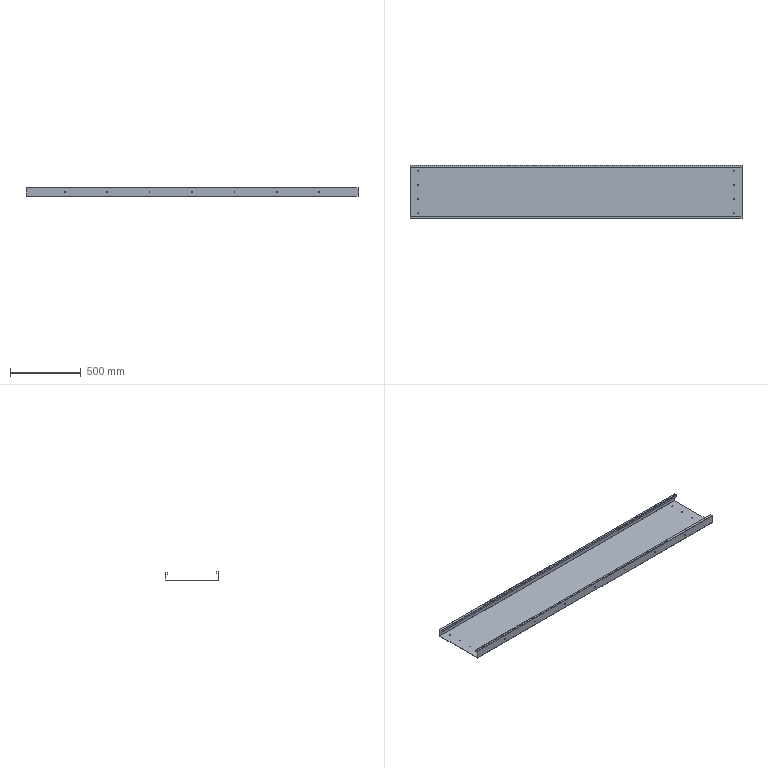Part | STEP file | TS-S15 | 1 solid | 98 faces | box 2350 x 380 x 62 mm | volume 2592719 mm3 | cylinder 56 | plane 42 | commonest cylinder face diameters 5.4 x28 7 x16 0.4 x6 4.4 x6